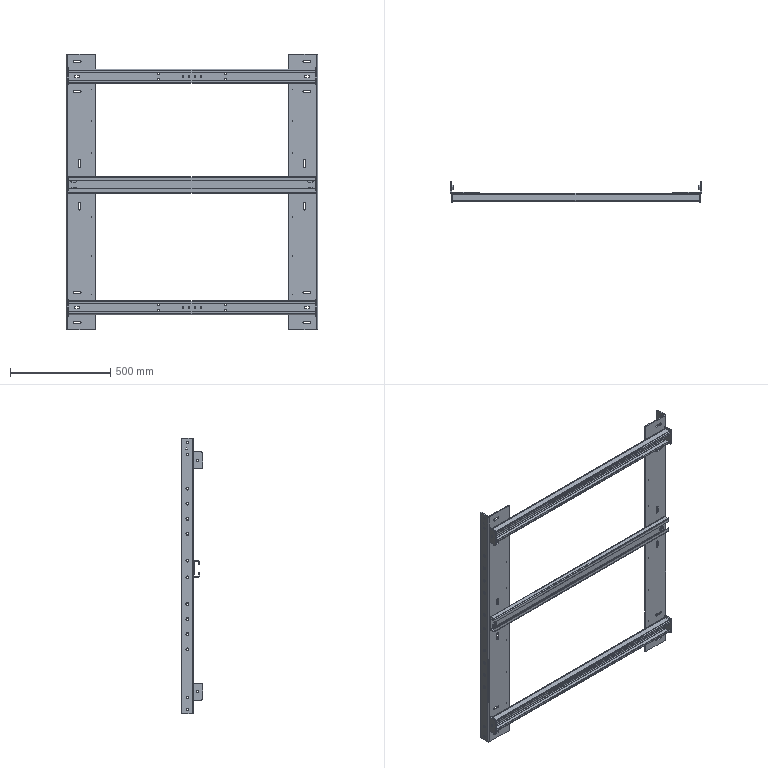Part | SolidWorks | features ReferencePattern 8, MirrorCompFeat 2 | 29 solids | 964 faces | box 1250 x 105 x 1370 mm | volume 4883387 mm3 | plane 512 | cylinder 332 | cone 120 | commonest cylinder face diameters 10.647 x40 14.75 x40 15 x40 15.07 x40 11 x32 13 x28